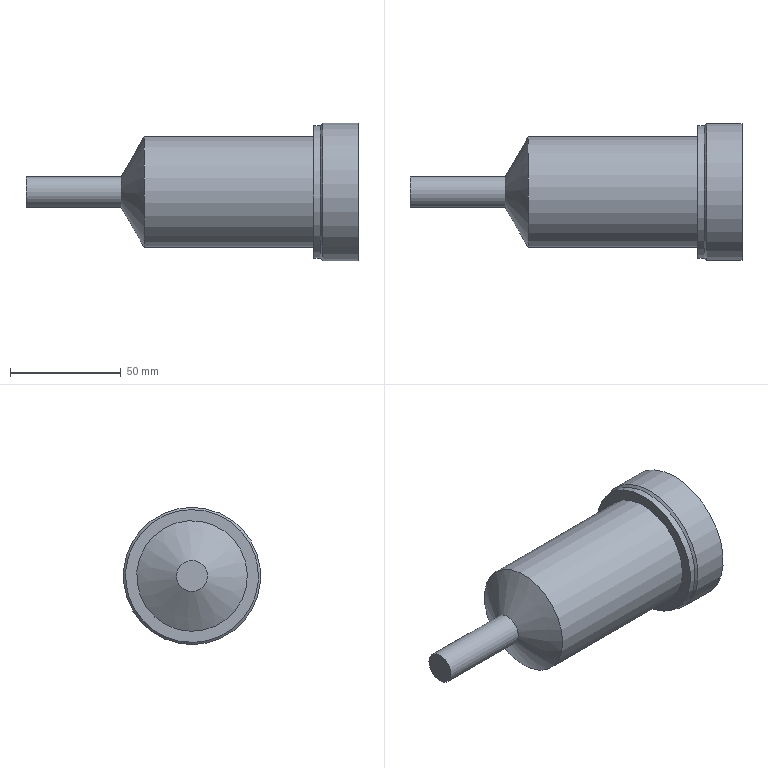Part | STEP file | 1-1 | 1 solid | 9 faces | box 150 x 62 x 62 mm | volume 225988 mm3 | cylinder 4 | plane 3 | cone 2 | commonest cylinder face diameters 14 x1 50 x1 60 x1 62 x1